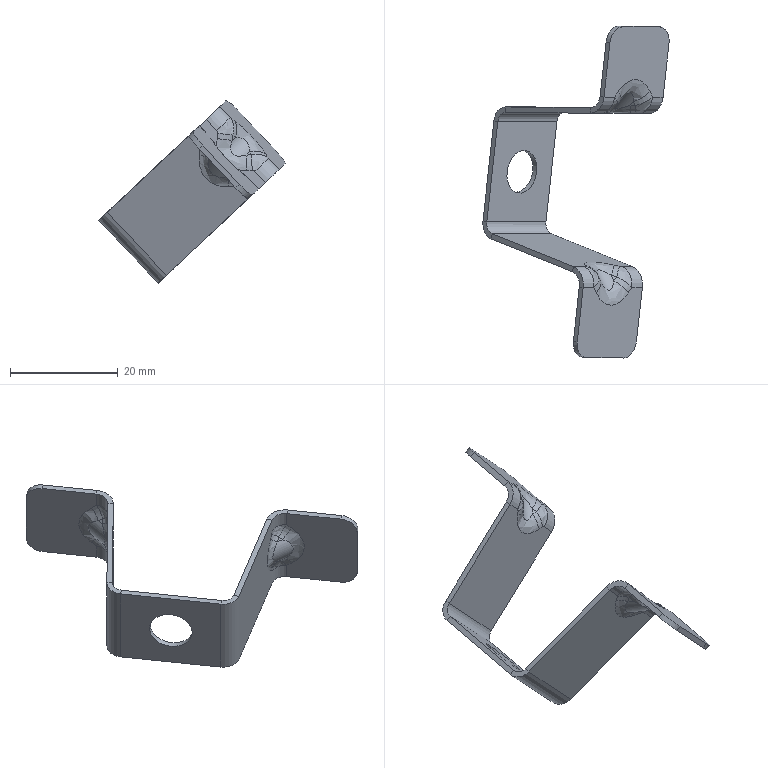Part | STEP file | FNA5401711 | 1 solid | 92 faces | box 34.513 x 61.465 x 33.785 mm | volume 1594 mm3 | cylinder 38 | spline 34 | plane 20 | commonest cylinder face diameters 6 x12 5 x8 7 x8 8 x8 4 x2